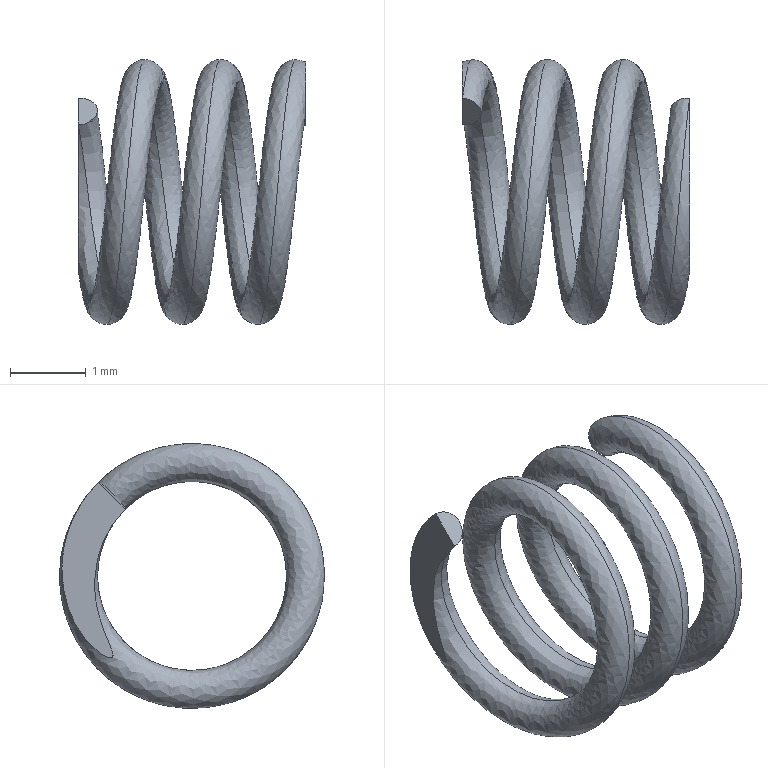Part | SolidWorks | features Helix 1, ICE 1, Sweep 1 | 1 solid | 6 faces | box 3 x 3.5 x 3.5 mm | volume 5.382 mm3 | plane 4 | spline 2
STEP:
#1=CARTESIAN_POINT('',(0.,1.237,1.237));
#2=VERTEX_POINT('',#1);
#3=CARTESIAN_POINT('',(0.,0.8839,0.8839));
#4=VERTEX_POINT('',#3);
#5=CARTESIAN_POINT('',(0.,1.061,1.061));
#6=DIRECTION('',(0.1055,0.7032,-0.7032));
#7=DIRECTION('',(0.,0.7071,0.7071));
#8=AXIS2_PLACEMENT_3D('',#5,#6,#7);
#9=CIRCLE('',#8,0.25);
#10=EDGE_CURVE('',#2,#4,#9,.T.);
#11=ORIENTED_EDGE('',*,*,#10,.T.);
#12=CARTESIAN_POINT('',(3.,0.8839,0.8839));
#13=VERTEX_POINT('',#12);
#14=CARTESIAN_POINT('',(0.,0.8839,0.8839));
#15=CARTESIAN_POINT('',(0.0625,1.25,0.5178));
#16=CARTESIAN_POINT('',(0.125,1.25,0.));
#17=CARTESIAN_POINT('',(0.1875,1.25,-0.5178));
#18=CARTESIAN_POINT('',(0.25,0.8839,-0.8839));
#19=CARTESIAN_POINT('',(0.3125,0.5178,-1.25));
#20=CARTESIAN_POINT('',(0.375,0.,-1.25));
#21=CARTESIAN_POINT('',(0.4375,-0.5178,-1.25));
#22=CARTESIAN_POINT('',(0.5,-0.8839,-0.8839));
#23=CARTESIAN_POINT('',(0.5625,-1.25,-0.5178));
#24=CARTESIAN_POINT('',(0.625,-1.25,0.));
#25=CARTESIAN_POINT('',(0.6875,-1.25,0.5178));
#26=CARTESIAN_POINT('',(0.75,-0.8839,0.8839));
#27=CARTESIAN_POINT('',(0.8125,-0.5178,1.25));
#28=CARTESIAN_POINT('',(0.875,0.,1.25));
#29=CARTESIAN_POINT('',(0.9375,0.5178,1.25));
#30=CARTESIAN_POINT('',(1.,0.8839,0.8839));
#31=CARTESIAN_POINT('',(1.063,1.25,0.5178));
#32=CARTESIAN_POINT('',(1.125,1.25,0.));
#33=CARTESIAN_POINT('',(1.188,1.25,-0.5178));
#34=CARTESIAN_POINT('',(1.25,0.8839,-0.8839));
#35=CARTESIAN_POINT('',(1.313,0.5178,-1.25));
#36=CARTESIAN_POINT('',(1.375,0.,-1.25));
#37=CARTESIAN_POINT('',(1.438,-0.5178,-1.25));
#38=CARTESIAN_POINT('',(1.5,-0.8839,-0.8839));
#39=CARTESIAN_POINT('',(1.562,-1.25,-0.5178));
#40=CARTESIAN_POINT('',(1.625,-1.25,0.));
#41=CARTESIAN_POINT('',(1.688,-1.25,0.5178));
#42=CARTESIAN_POINT('',(1.75,-0.8839,0.8839));
#43=CARTESIAN_POINT('',(1.812,-0.5178,1.25));
#44=CARTESIAN_POINT('',(1.875,0.,1.25));
#45=CARTESIAN_POINT('',(1.938,0.5178,1.25));
#46=CARTESIAN_POINT('',(2.,0.8839,0.8839));
#47=CARTESIAN_POINT('',(2.062,1.25,0.5178));
#48=CARTESIAN_POINT('',(2.125,1.25,0.));
#49=CARTESIAN_POINT('',(2.188,1.25,-0.5178));
#50=CARTESIAN_POINT('',(2.25,0.8839,-0.8839));
#51=CARTESIAN_POINT('',(2.313,0.5178,-1.25));
#52=CARTESIAN_POINT('',(2.375,0.,-1.25));
#53=CARTESIAN_POINT('',(2.438,-0.5178,-1.25));
#54=CARTESIAN_POINT('',(2.5,-0.8839,-0.8839));
#55=CARTESIAN_POINT('',(2.563,-1.25,-0.5178));
#56=CARTESIAN_POINT('',(2.625,-1.25,0.));
#57=CARTESIAN_POINT('',(2.688,-1.25,0.5178));
#58=CARTESIAN_POINT('',(2.75,-0.8839,0.8839));
#59=CARTESIAN_POINT('',(2.812,-0.5178,1.25));
#60=CARTESIAN_POINT('',(2.875,0.,1.25));
#61=CARTESIAN_POINT('',(2.938,0.5178,1.25));
#62=CARTESIAN_POINT('',(3.,0.8839,0.8839));
#63=(BOUNDED_CURVE()B_SPLINE_CURVE(2,(#14,#15,#16,#17,#18,#19,#20,#21,#22,#23,#24,#25,#26,#27,#28,#29,#30,#31,#32,#33,#34,#35,#36,#37,#38,#39,#40,#41,#42,#43,#44,#45,#46,#47,#48,#49,#50,#51,#52,#53,#54,#55,#56,#57,#58,#59,#60,#61,#62),.UNSPECIFIED.,.F.,.T.)B_SPLINE_CURVE_WITH_KNOTS((3,2,2,2,2,2,2,2,2,2,2,2,2,2,2,2,2,2,2,2,2,2,2,2,3),(0.,0.04167,0.08333,0.125,0.1667,0.2083,0.25,0.2917,0.3333,0.375,0.4167,0.4583,0.5,0.5417,0.5833,0.625,0.6667,0.7083,0.75,0.7917,0.8333,0.875,0.9167,0.9583,1.),.UNSPECIFIED.)CURVE()GEOMETRIC_REPRESENTATION_ITEM()RATIONAL_B_SPLINE_CURVE((1.,0.9239,1.,0.9239,1.,0.9239,1.,0.9239,1.,0.9239,1.,0.9239,1.,0.9239,1.,0.9239,1.,0.9239,1.,0.9239,1.,0.9239,1.,0.9239,1.,0.9239,1.,0.9239,1.,0.9239,1.,0.9239,1.,0.9239,1.,0.9239,1.,0.9239,1.,0.9239,1.,0.9239,1.,0.9239,1.,0.9239,1.,0.9239,1.))REPRESENTATION_ITEM(''));
#64=EDGE_CURVE('',#4,#13,#63,.T.);
#65=ORIENTED_EDGE('',*,*,#64,.T.);
#66=CARTESIAN_POINT('',(3.,1.237,1.237));
#67=VERTEX_POINT('',#66);
#68=CARTESIAN_POINT('',(3.,0.8839,0.8839));
#69=CARTESIAN_POINT('',(3.,0.8117,0.956));
#70=CARTESIAN_POINT('',(3.,0.7329,1.019));
#71=CARTESIAN_POINT('',(3.,0.5624,1.126));
#72=CARTESIAN_POINT('',(3.,0.4699,1.171));
#73=CARTESIAN_POINT('',(3.,0.1851,1.273));
#74=CARTESIAN_POINT('',(3.,-0.02075,1.298));
#75=CARTESIAN_POINT('',(3.,-0.3223,1.273));
#76=CARTESIAN_POINT('',(3.,-0.4231,1.255));
#77=CARTESIAN_POINT('',(3.,-0.6187,1.203));
#78=CARTESIAN_POINT('',(3.,-0.7141,1.167));
#79=CARTESIAN_POINT('',(3.,-0.8547,1.108));
#80=CARTESIAN_POINT('',(3.,-0.901,1.087));
#81=CARTESIAN_POINT('',(3.,-0.9719,1.059));
#82=CARTESIAN_POINT('',(3.,-0.9959,1.05));
#83=CARTESIAN_POINT('',(3.,-1.033,1.043));
#84=CARTESIAN_POINT('',(3.,-1.046,1.041));
#85=CARTESIAN_POINT('',(3.,-1.071,1.049));
#86=CARTESIAN_POINT('',(3.,-1.078,1.062));
#87=CARTESIAN_POINT('',(3.,-1.079,1.101));
#88=CARTESIAN_POINT('',(3.,-1.068,1.125));
#89=CARTESIAN_POINT('',(3.,-1.046,1.17));
#90=CARTESIAN_POINT('',(3.,-1.033,1.192));
#91=CARTESIAN_POINT('',(3.,-0.9907,1.254));
#92=CARTESIAN_POINT('',(3.,-0.9577,1.292));
#93=CARTESIAN_POINT('',(3.,-0.8525,1.398));
#94=CARTESIAN_POINT('',(3.,-0.7724,1.46));
#95=CARTESIAN_POINT('',(3.,-0.6013,1.563));
#96=CARTESIAN_POINT('',(3.,-0.5113,1.605));
#97=CARTESIAN_POINT('',(3.,-0.3232,1.669));
#98=CARTESIAN_POINT('',(3.,-0.2247,1.692));
#99=CARTESIAN_POINT('',(3.,-0.02778,1.718));
#100=CARTESIAN_POINT('',(3.,0.07173,1.722));
#101=CARTESIAN_POINT('',(3.,0.3722,1.705));
#102=CARTESIAN_POINT('',(3.,0.5671,1.657));
#103=CARTESIAN_POINT('',(3.,0.9306,1.493));
#104=CARTESIAN_POINT('',(3.,1.096,1.379));
#105=CARTESIAN_POINT('',(3.,1.237,1.237));
#106=B_SPLINE_CURVE_WITH_KNOTS('',3,(#68,#69,#70,#71,#72,#73,#74,#75,#76,#77,#78,#79,#80,#81,#82,#83,#84,#85,#86,#87,#88,#89,#90,#91,#92,#93,#94,#95,#96,#97,#98,#99,#100,#101,#102,#103,#104,#105),.UNSPECIFIED.,.F.,.F.,(4,2,2,2,2,2,2,2,2,2,2,2,2,2,2,2,2,2,4),(0.,0.0003018,0.0006036,0.001207,0.001509,0.001811,0.001962,0.002037,0.002075,0.002113,0.002188,0.002263,0.002414,0.002716,0.003018,0.00332,0.003622,0.004225,0.004829),.UNSPECIFIED.);
#107=EDGE_CURVE('',#13,#67,#106,.T.);
#108=ORIENTED_EDGE('',*,*,#107,.T.);
#109=CARTESIAN_POINT('',(0.,1.237,1.237));
#110=CARTESIAN_POINT('',(0.0625,1.75,0.7249));
#111=CARTESIAN_POINT('',(0.125,1.75,0.));
#112=CARTESIAN_POINT('',(0.1875,1.75,-0.7249));
#113=CARTESIAN_POINT('',(0.25,1.237,-1.237));
#114=CARTESIAN_POINT('',(0.3125,0.7249,-1.75));
#115=CARTESIAN_POINT('',(0.375,0.,-1.75));
#116=CARTESIAN_POINT('',(0.4375,-0.7249,-1.75));
#117=CARTESIAN_POINT('',(0.5,-1.237,-1.237));
#118=CARTESIAN_POINT('',(0.5625,-1.75,-0.7249));
#119=CARTESIAN_POINT('',(0.625,-1.75,0.));
#120=CARTESIAN_POINT('',(0.6875,-1.75,0.7249));
#121=CARTESIAN_POINT('',(0.75,-1.237,1.237));
#122=CARTESIAN_POINT('',(0.8125,-0.7249,1.75));
#123=CARTESIAN_POINT('',(0.875,0.,1.75));
#124=CARTESIAN_POINT('',(0.9375,0.7249,1.75));
#125=CARTESIAN_POINT('',(1.,1.237,1.237));
#126=CARTESIAN_POINT('',(1.063,1.75,0.7249));
#127=CARTESIAN_POINT('',(1.125,1.75,0.));
#128=CARTESIAN_POINT('',(1.188,1.75,-0.7249));
#129=CARTESIAN_POINT('',(1.25,1.237,-1.237));
#130=CARTESIAN_POINT('',(1.313,0.7249,-1.75));
#131=CARTESIAN_POINT('',(1.375,0.,-1.75));
#132=CARTESIAN_POINT('',(1.438,-0.7249,-1.75));
#133=CARTESIAN_POINT('',(1.5,-1.237,-1.237));
#134=CARTESIAN_POINT('',(1.562,-1.75,-0.7249));
#135=CARTESIAN_POINT('',(1.625,-1.75,0.));
#136=CARTESIAN_POINT('',(1.688,-1.75,0.7249));
#137=CARTESIAN_POINT('',(1.75,-1.237,1.237));
#138=CARTESIAN_POINT('',(1.812,-0.7249,1.75));
#139=CARTESIAN_POINT('',(1.875,0.,1.75));
#140=CARTESIAN_POINT('',(1.938,0.7249,1.75));
#141=CARTESIAN_POINT('',(2.,1.237,1.237));
#142=CARTESIAN_POINT('',(2.062,1.75,0.7249));
#143=CARTESIAN_POINT('',(2.125,1.75,0.));
#144=CARTESIAN_POINT('',(2.188,1.75,-0.7249));
#145=CARTESIAN_POINT('',(2.25,1.237,-1.237));
#146=CARTESIAN_POINT('',(2.313,0.7249,-1.75));
#147=CARTESIAN_POINT('',(2.375,0.,-1.75));
#148=CARTESIAN_POINT('',(2.438,-0.7249,-1.75));
#149=CARTESIAN_POINT('',(2.5,-1.237,-1.237));
#150=CARTESIAN_POINT('',(2.563,-1.75,-0.7249));
#151=CARTESIAN_POINT('',(2.625,-1.75,0.));
#152=CARTESIAN_POINT('',(2.688,-1.75,0.7249));
#153=CARTESIAN_POINT('',(2.75,-1.237,1.237));
#154=CARTESIAN_POINT('',(2.812,-0.7249,1.75));
#155=CARTESIAN_POINT('',(2.875,0.,1.75));
#156=CARTESIAN_POINT('',(2.938,0.7249,1.75));
#157=CARTESIAN_POINT('',(3.,1.237,1.237));
#158=(BOUNDED_CURVE()B_SPLINE_CURVE(2,(#109,#110,#111,#112,#113,#114,#115,#116,#117,#118,#119,#120,#121,#122,#123,#124,#125,#126,#127,#128,#129,#130,#131,#132,#133,#134,#135,#136,#137,#138,#139,#140,#141,#142,#143,#144,#145,#146,#147,#148,#149,#150,#151,#152,#153,#154,#155,#156,#157),.UNSPECIFIED.,.F.,.T.)B_SPLINE_CURVE_WITH_KNOTS((3,2,2,2,2,2,2,2,2,2,2,2,2,2,2,2,2,2,2,2,2,2,2,2,3),(0.,0.04167,0.08333,0.125,0.1667,0.2083,0.25,0.2917,0.3333,0.375,0.4167,0.4583,0.5,0.5417,0.5833,0.625,0.6667,0.7083,0.75,0.7917,0.8333,0.875,0.9167,0.9583,1.),.UNSPECIFIED.)CURVE()GEOMETRIC_REPRESENTATION_ITEM()RATIONAL_B_SPLINE_CURVE((1.,0.9239,1.,0.9239,1.,0.9239,1.,0.9239,1.,0.9239,1.,0.9239,1.,0.9239,1.,0.9239,1.,0.9239,1.,0.9239,1.,0.9239,1.,0.9239,1.,0.9239,1.,0.9239,1.,0.9239,1.,0.9239,1.,0.9239,1.,0.9239,1.,0.9239,1.,0.9239,1.,0.9239,1.,0.9239,1.,0.9239,1.,0.9239,1.))REPRESENTATION_ITEM(''));
#159=EDGE_CURVE('',#2,#67,#158,.T.);
#160=ORIENTED_EDGE('',*,*,#159,.F.);
#161=EDGE_LOOP('',(#11,#65,#108,#160));
#162=FACE_OUTER_BOUND('',#161,.T.);
#163=CARTESIAN_POINT('',(0.,1.237,1.237));
#164=CARTESIAN_POINT('',(0.0625,1.75,0.7249));
#165=CARTESIAN_POINT('',(0.125,1.75,0.));
#166=CARTESIAN_POINT('',(0.1875,1.75,-0.7249));
#167=CARTESIAN_POINT('',(0.25,1.237,-1.237));
#168=CARTESIAN_POINT('',(0.3125,0.7249,-1.75));
#169=CARTESIAN_POINT('',(0.375,0.,-1.75));
#170=CARTESIAN_POINT('',(0.4375,-0.7249,-1.75));
#171=CARTESIAN_POINT('',(0.5,-1.237,-1.237));
#172=CARTESIAN_POINT('',(0.5625,-1.75,-0.7249));
#173=CARTESIAN_POINT('',(0.625,-1.75,0.));
#174=CARTESIAN_POINT('',(0.6875,-1.75,0.7249));
#175=CARTESIAN_POINT('',(0.75,-1.237,1.237));
#176=CARTESIAN_POINT('',(0.8125,-0.7249,1.75));
#177=CARTESIAN_POINT('',(0.875,0.,1.75));
#178=CARTESIAN_POINT('',(0.9375,0.7249,1.75));
#179=CARTESIAN_POINT('',(1.,1.237,1.237));
#180=CARTESIAN_POINT('',(1.063,1.75,0.7249));
#181=CARTESIAN_POINT('',(1.125,1.75,0.));
#182=CARTESIAN_POINT('',(1.188,1.75,-0.7249));
#183=CARTESIAN_POINT('',(1.25,1.237,-1.237));
#184=CARTESIAN_POINT('',(1.313,0.7249,-1.75));
#185=CARTESIAN_POINT('',(1.375,0.,-1.75));
#186=CARTESIAN_POINT('',(1.438,-0.7249,-1.75));
#187=CARTESIAN_POINT('',(1.5,-1.237,-1.237));
#188=CARTESIAN_POINT('',(1.562,-1.75,-0.7249));
#189=CARTESIAN_POINT('',(1.625,-1.75,0.));
#190=CARTESIAN_POINT('',(1.688,-1.75,0.7249));
#191=CARTESIAN_POINT('',(1.75,-1.237,1.237));
#192=CARTESIAN_POINT('',(1.813,-0.7249,1.75));
#193=CARTESIAN_POINT('',(1.875,0.,1.75));
#194=CARTESIAN_POINT('',(1.938,0.7249,1.75));
#195=CARTESIAN_POINT('',(2.,1.237,1.237));
#196=CARTESIAN_POINT('',(2.062,1.75,0.7249));
#197=CARTESIAN_POINT('',(2.125,1.75,0.));
#198=CARTESIAN_POINT('',(2.188,1.75,-0.7249));
#199=CARTESIAN_POINT('',(2.25,1.237,-1.237));
#200=CARTESIAN_POINT('',(2.313,0.7249,-1.75));
#201=CARTESIAN_POINT('',(2.375,0.,-1.75));
#202=CARTESIAN_POINT('',(2.438,-0.7249,-1.75));
#203=CARTESIAN_POINT('',(2.5,-1.237,-1.237));
#204=CARTESIAN_POINT('',(2.563,-1.75,-0.7249));
#205=CARTESIAN_POINT('',(2.625,-1.75,0.));
#206=CARTESIAN_POINT('',(2.688,-1.75,0.7249));
#207=CARTESIAN_POINT('',(2.75,-1.237,1.237));
#208=CARTESIAN_POINT('',(2.812,-0.7249,1.75));
#209=CARTESIAN_POINT('',(2.875,0.,1.75));
#210=CARTESIAN_POINT('',(2.938,0.7249,1.75));
#211=CARTESIAN_POINT('',(3.,1.237,1.237));
#212=CARTESIAN_POINT('',(0.4972,1.2,1.275));
#213=CARTESIAN_POINT('',(0.5597,1.728,0.7776));
#214=CARTESIAN_POINT('',(0.6222,1.75,0.05276));
#215=CARTESIAN_POINT('',(0.6847,1.772,-0.6721));
#216=CARTESIAN_POINT('',(0.7472,1.275,-1.2));
#217=CARTESIAN_POINT('',(0.8097,0.7776,-1.728));
#218=CARTESIAN_POINT('',(0.8722,0.05276,-1.75));
#219=CARTESIAN_POINT('',(0.9347,-0.6721,-1.772));
#220=CARTESIAN_POINT('',(0.9972,-1.2,-1.275));
#221=CARTESIAN_POINT('',(1.06,-1.728,-0.7776));
#222=CARTESIAN_POINT('',(1.122,-1.75,-0.05276));
#223=CARTESIAN_POINT('',(1.185,-1.772,0.6721));
#224=CARTESIAN_POINT('',(1.247,-1.275,1.2));
#225=CARTESIAN_POINT('',(1.31,-0.7776,1.728));
#226=CARTESIAN_POINT('',(1.372,-0.05276,1.75));
#227=CARTESIAN_POINT('',(1.435,0.6721,1.772));
#228=CARTESIAN_POINT('',(1.497,1.2,1.275));
#229=CARTESIAN_POINT('',(1.56,1.728,0.7776));
#230=CARTESIAN_POINT('',(1.622,1.75,0.05276));
#231=CARTESIAN_POINT('',(1.685,1.772,-0.6721));
#232=CARTESIAN_POINT('',(1.747,1.275,-1.2));
#233=CARTESIAN_POINT('',(1.81,0.7776,-1.728));
#234=CARTESIAN_POINT('',(1.872,0.05276,-1.75));
#235=CARTESIAN_POINT('',(1.935,-0.6721,-1.772));
#236=CARTESIAN_POINT('',(1.997,-1.2,-1.275));
#237=CARTESIAN_POINT('',(2.06,-1.728,-0.7776));
#238=CARTESIAN_POINT('',(2.122,-1.75,-0.05276));
#239=CARTESIAN_POINT('',(2.185,-1.772,0.6721));
#240=CARTESIAN_POINT('',(2.247,-1.275,1.2));
#241=CARTESIAN_POINT('',(2.31,-0.7776,1.728));
#242=CARTESIAN_POINT('',(2.372,-0.05276,1.75));
#243=CARTESIAN_POINT('',(2.435,0.6721,1.772));
#244=CARTESIAN_POINT('',(2.497,1.2,1.275));
#245=CARTESIAN_POINT('',(2.56,1.728,0.7776));
#246=CARTESIAN_POINT('',(2.622,1.75,0.05276));
#247=CARTESIAN_POINT('',(2.685,1.772,-0.6721));
#248=CARTESIAN_POINT('',(2.747,1.275,-1.2));
#249=CARTESIAN_POINT('',(2.81,0.7776,-1.728));
#250=CARTESIAN_POINT('',(2.872,0.05276,-1.75));
#251=CARTESIAN_POINT('',(2.935,-0.6721,-1.772));
#252=CARTESIAN_POINT('',(2.997,-1.2,-1.275));
#253=CARTESIAN_POINT('',(3.06,-1.728,-0.7776));
#254=CARTESIAN_POINT('',(3.122,-1.75,-0.05276));
#255=CARTESIAN_POINT('',(3.185,-1.772,0.6721));
#256=CARTESIAN_POINT('',(3.247,-1.275,1.2));
#257=CARTESIAN_POINT('',(3.31,-0.7776,1.728));
#258=CARTESIAN_POINT('',(3.372,-0.05276,1.75));
#259=CARTESIAN_POINT('',(3.435,0.6721,1.772));
#260=CARTESIAN_POINT('',(3.497,1.2,1.275));
#261=CARTESIAN_POINT('',(0.4972,0.8466,0.9212));
#262=CARTESIAN_POINT('',(0.5597,1.228,0.5705));
#263=CARTESIAN_POINT('',(0.6222,1.25,0.05276));
#264=CARTESIAN_POINT('',(0.6847,1.272,-0.465));
#265=CARTESIAN_POINT('',(0.7472,0.9212,-0.8466));
#266=CARTESIAN_POINT('',(0.8097,0.5705,-1.228));
#267=CARTESIAN_POINT('',(0.8722,0.05276,-1.25));
#268=CARTESIAN_POINT('',(0.9347,-0.465,-1.272));
#269=CARTESIAN_POINT('',(0.9972,-0.8466,-0.9212));
#270=CARTESIAN_POINT('',(1.06,-1.228,-0.5705));
#271=CARTESIAN_POINT('',(1.122,-1.25,-0.05276));
#272=CARTESIAN_POINT('',(1.185,-1.272,0.465));
#273=CARTESIAN_POINT('',(1.247,-0.9212,0.8466));
#274=CARTESIAN_POINT('',(1.31,-0.5705,1.228));
#275=CARTESIAN_POINT('',(1.372,-0.05276,1.25));
#276=CARTESIAN_POINT('',(1.435,0.465,1.272));
#277=CARTESIAN_POINT('',(1.497,0.8466,0.9212));
#278=CARTESIAN_POINT('',(1.56,1.228,0.5705));
#279=CARTESIAN_POINT('',(1.622,1.25,0.05276));
#280=CARTESIAN_POINT('',(1.685,1.272,-0.465));
#281=CARTESIAN_POINT('',(1.747,0.9212,-0.8466));
#282=CARTESIAN_POINT('',(1.81,0.5705,-1.228));
#283=CARTESIAN_POINT('',(1.872,0.05276,-1.25));
#284=CARTESIAN_POINT('',(1.935,-0.465,-1.272));
#285=CARTESIAN_POINT('',(1.997,-0.8466,-0.9212));
#286=CARTESIAN_POINT('',(2.06,-1.228,-0.5705));
#287=CARTESIAN_POINT('',(2.122,-1.25,-0.05276));
#288=CARTESIAN_POINT('',(2.185,-1.272,0.465));
#289=CARTESIAN_POINT('',(2.247,-0.9212,0.8466));
#290=CARTESIAN_POINT('',(2.31,-0.5705,1.228));
#291=CARTESIAN_POINT('',(2.372,-0.05276,1.25));
#292=CARTESIAN_POINT('',(2.435,0.465,1.272));
#293=CARTESIAN_POINT('',(2.497,0.8466,0.9212));
#294=CARTESIAN_POINT('',(2.56,1.228,0.5705));
#295=CARTESIAN_POINT('',(2.622,1.25,0.05276));
#296=CARTESIAN_POINT('',(2.685,1.272,-0.465));
#297=CARTESIAN_POINT('',(2.747,0.9212,-0.8466));
#298=CARTESIAN_POINT('',(2.81,0.5705,-1.228));
#299=CARTESIAN_POINT('',(2.872,0.05276,-1.25));
#300=CARTESIAN_POINT('',(2.935,-0.465,-1.272));
#301=CARTESIAN_POINT('',(2.997,-0.8466,-0.9212));
#302=CARTESIAN_POINT('',(3.06,-1.228,-0.5705));
#303=CARTESIAN_POINT('',(3.122,-1.25,-0.05276));
#304=CARTESIAN_POINT('',(3.185,-1.272,0.465));
#305=CARTESIAN_POINT('',(3.247,-0.9212,0.8466));
#306=CARTESIAN_POINT('',(3.31,-0.5705,1.228));
#307=CARTESIAN_POINT('',(3.372,-0.05276,1.25));
#308=CARTESIAN_POINT('',(3.435,0.465,1.272));
#309=CARTESIAN_POINT('',(3.497,0.8466,0.9212));
#310=CARTESIAN_POINT('',(0.,0.8839,0.8839));
#311=CARTESIAN_POINT('',(0.0625,1.25,0.5178));
#312=CARTESIAN_POINT('',(0.125,1.25,0.));
#313=CARTESIAN_POINT('',(0.1875,1.25,-0.5178));
#314=CARTESIAN_POINT('',(0.25,0.8839,-0.8839));
#315=CARTESIAN_POINT('',(0.3125,0.5178,-1.25));
#316=CARTESIAN_POINT('',(0.375,0.,-1.25));
#317=CARTESIAN_POINT('',(0.4375,-0.5178,-1.25));
#318=CARTESIAN_POINT('',(0.5,-0.8839,-0.8839));
#319=CARTESIAN_POINT('',(0.5625,-1.25,-0.5178));
#320=CARTESIAN_POINT('',(0.625,-1.25,0.));
#321=CARTESIAN_POINT('',(0.6875,-1.25,0.5178));
#322=CARTESIAN_POINT('',(0.75,-0.8839,0.8839));
#323=CARTESIAN_POINT('',(0.8125,-0.5178,1.25));
#324=CARTESIAN_POINT('',(0.875,0.,1.25));
#325=CARTESIAN_POINT('',(0.9375,0.5178,1.25));
#326=CARTESIAN_POINT('',(1.,0.8839,0.8839));
#327=CARTESIAN_POINT('',(1.063,1.25,0.5178));
#328=CARTESIAN_POINT('',(1.125,1.25,0.));
#329=CARTESIAN_POINT('',(1.188,1.25,-0.5178));
#330=CARTESIAN_POINT('',(1.25,0.8839,-0.8839));
#331=CARTESIAN_POINT('',(1.313,0.5178,-1.25));
#332=CARTESIAN_POINT('',(1.375,0.,-1.25));
#333=CARTESIAN_POINT('',(1.438,-0.5178,-1.25));
#334=CARTESIAN_POINT('',(1.5,-0.8839,-0.8839));
#335=CARTESIAN_POINT('',(1.562,-1.25,-0.5178));
#336=CARTESIAN_POINT('',(1.625,-1.25,0.));
#337=CARTESIAN_POINT('',(1.688,-1.25,0.5178));
#338=CARTESIAN_POINT('',(1.75,-0.8839,0.8839));
#339=CARTESIAN_POINT('',(1.813,-0.5178,1.25));
#340=CARTESIAN_POINT('',(1.875,0.,1.25));
#341=CARTESIAN_POINT('',(1.938,0.5178,1.25));
#342=CARTESIAN_POINT('',(2.,0.8839,0.8839));
#343=CARTESIAN_POINT('',(2.062,1.25,0.5178));
#344=CARTESIAN_POINT('',(2.125,1.25,0.));
#345=CARTESIAN_POINT('',(2.188,1.25,-0.5178));
#346=CARTESIAN_POINT('',(2.25,0.8839,-0.8839));
#347=CARTESIAN_POINT('',(2.313,0.5178,-1.25));
#348=CARTESIAN_POINT('',(2.375,0.,-1.25));
#349=CARTESIAN_POINT('',(2.438,-0.5178,-1.25));
#350=CARTESIAN_POINT('',(2.5,-0.8839,-0.8839));
#351=CARTESIAN_POINT('',(2.563,-1.25,-0.5178));
#352=CARTESIAN_POINT('',(2.625,-1.25,0.));
#353=CARTESIAN_POINT('',(2.688,-1.25,0.5178));
#354=CARTESIAN_POINT('',(2.75,-0.8839,0.8839));
#355=CARTESIAN_POINT('',(2.812,-0.5178,1.25));
#356=CARTESIAN_POINT('',(2.875,0.,1.25));
#357=CARTESIAN_POINT('',(2.938,0.5178,1.25));
#358=CARTESIAN_POINT('',(3.,0.8839,0.8839));
#359=CARTESIAN_POINT('',(-0.4972,0.9212,0.8466));
#360=CARTESIAN_POINT('',(-0.4347,1.272,0.465));
#361=CARTESIAN_POINT('',(-0.3722,1.25,-0.05276));
#362=CARTESIAN_POINT('',(-0.3097,1.228,-0.5705));
#363=CARTESIAN_POINT('',(-0.2472,0.8466,-0.9212));
#364=CARTESIAN_POINT('',(-0.1847,0.465,-1.272));
#365=CARTESIAN_POINT('',(-0.1222,-0.05276,-1.25));
#366=CARTESIAN_POINT('',(-0.05971,-0.5705,-1.228));
#367=CARTESIAN_POINT('',(0.002791,-0.9212,-0.8466));
#368=CARTESIAN_POINT('',(0.06529,-1.272,-0.465));
#369=CARTESIAN_POINT('',(0.1278,-1.25,0.05276));
#370=CARTESIAN_POINT('',(0.1903,-1.228,0.5705));
#371=CARTESIAN_POINT('',(0.2528,-0.8466,0.9212));
#372=CARTESIAN_POINT('',(0.3153,-0.465,1.272));
#373=CARTESIAN_POINT('',(0.3778,0.05276,1.25));
#374=CARTESIAN_POINT('',(0.4403,0.5705,1.228));
#375=CARTESIAN_POINT('',(0.5028,0.9212,0.8466));
#376=CARTESIAN_POINT('',(0.5653,1.272,0.465));
#377=CARTESIAN_POINT('',(0.6278,1.25,-0.05276));
#378=CARTESIAN_POINT('',(0.6903,1.228,-0.5705));
#379=CARTESIAN_POINT('',(0.7528,0.8466,-0.9212));
#380=CARTESIAN_POINT('',(0.8153,0.465,-1.272));
#381=CARTESIAN_POINT('',(0.8778,-0.05276,-1.25));
#382=CARTESIAN_POINT('',(0.9403,-0.5705,-1.228));
#383=CARTESIAN_POINT('',(1.003,-0.9212,-0.8466));
#384=CARTESIAN_POINT('',(1.065,-1.272,-0.465));
#385=CARTESIAN_POINT('',(1.128,-1.25,0.05276));
#386=CARTESIAN_POINT('',(1.19,-1.228,0.5705));
#387=CARTESIAN_POINT('',(1.253,-0.8466,0.9212));
#388=CARTESIAN_POINT('',(1.315,-0.465,1.272));
#389=CARTESIAN_POINT('',(1.378,0.05276,1.25));
#390=CARTESIAN_POINT('',(1.44,0.5705,1.228));
#391=CARTESIAN_POINT('',(1.503,0.9212,0.8466));
#392=CARTESIAN_POINT('',(1.565,1.272,0.465));
#393=CARTESIAN_POINT('',(1.628,1.25,-0.05276));
#394=CARTESIAN_POINT('',(1.69,1.228,-0.5705));
#395=CARTESIAN_POINT('',(1.753,0.8466,-0.9212));
#396=CARTESIAN_POINT('',(1.815,0.465,-1.272));
#397=CARTESIAN_POINT('',(1.878,-0.05276,-1.25));
#398=CARTESIAN_POINT('',(1.94,-0.5705,-1.228));
#399=CARTESIAN_POINT('',(2.003,-0.9212,-0.8466));
#400=CARTESIAN_POINT('',(2.065,-1.272,-0.465));
#401=CARTESIAN_POINT('',(2.128,-1.25,0.05276));
#402=CARTESIAN_POINT('',(2.19,-1.228,0.5705));
#403=CARTESIAN_POINT('',(2.253,-0.8466,0.9212));
#404=CARTESIAN_POINT('',(2.315,-0.465,1.272));
#405=CARTESIAN_POINT('',(2.378,0.05276,1.25));
#406=CARTESIAN_POINT('',(2.44,0.5705,1.228));
#407=CARTESIAN_POINT('',(2.503,0.9212,0.8466));
#408=CARTESIAN_POINT('',(-0.4972,1.275,1.2));
#409=CARTESIAN_POINT('',(-0.4347,1.772,0.6721));
#410=CARTESIAN_POINT('',(-0.3722,1.75,-0.05276));
#411=CARTESIAN_POINT('',(-0.3097,1.728,-0.7776));
#412=CARTESIAN_POINT('',(-0.2472,1.2,-1.275));
#413=CARTESIAN_POINT('',(-0.1847,0.6721,-1.772));
#414=CARTESIAN_POINT('',(-0.1222,-0.05276,-1.75));
#415=CARTESIAN_POINT('',(-0.05971,-0.7776,-1.728));
#416=CARTESIAN_POINT('',(0.002791,-1.275,-1.2));
#417=CARTESIAN_POINT('',(0.06529,-1.772,-0.6721));
#418=CARTESIAN_POINT('',(0.1278,-1.75,0.05276));
#419=CARTESIAN_POINT('',(0.1903,-1.728,0.7776));
#420=CARTESIAN_POINT('',(0.2528,-1.2,1.275));
#421=CARTESIAN_POINT('',(0.3153,-0.6721,1.772));
#422=CARTESIAN_POINT('',(0.3778,0.05276,1.75));
#423=CARTESIAN_POINT('',(0.4403,0.7776,1.728));
#424=CARTESIAN_POINT('',(0.5028,1.275,1.2));
#425=CARTESIAN_POINT('',(0.5653,1.772,0.6721));
#426=CARTESIAN_POINT('',(0.6278,1.75,-0.05276));
#427=CARTESIAN_POINT('',(0.6903,1.728,-0.7776));
#428=CARTESIAN_POINT('',(0.7528,1.2,-1.275));
#429=CARTESIAN_POINT('',(0.8153,0.6721,-1.772));
#430=CARTESIAN_POINT('',(0.8778,-0.05276,-1.75));
#431=CARTESIAN_POINT('',(0.9403,-0.7776,-1.728));
#432=CARTESIAN_POINT('',(1.003,-1.275,-1.2));
#433=CARTESIAN_POINT('',(1.065,-1.772,-0.6721));
#434=CARTESIAN_POINT('',(1.128,-1.75,0.05276));
#435=CARTESIAN_POINT('',(1.19,-1.728,0.7776));
#436=CARTESIAN_POINT('',(1.253,-1.2,1.275));
#437=CARTESIAN_POINT('',(1.315,-0.6721,1.772));
#438=CARTESIAN_POINT('',(1.378,0.05276,1.75));
#439=CARTESIAN_POINT('',(1.44,0.7776,1.728));
#440=CARTESIAN_POINT('',(1.503,1.275,1.2));
#441=CARTESIAN_POINT('',(1.565,1.772,0.6721));
#442=CARTESIAN_POINT('',(1.628,1.75,-0.05276));
#443=CARTESIAN_POINT('',(1.69,1.728,-0.7776));
#444=CARTESIAN_POINT('',(1.753,1.2,-1.275));
#445=CARTESIAN_POINT('',(1.815,0.6721,-1.772));
#446=CARTESIAN_POINT('',(1.878,-0.05276,-1.75));
#447=CARTESIAN_POINT('',(1.94,-0.7776,-1.728));
#448=CARTESIAN_POINT('',(2.003,-1.275,-1.2));
#449=CARTESIAN_POINT('',(2.065,-1.772,-0.6721));
#450=CARTESIAN_POINT('',(2.128,-1.75,0.05276));
#451=CARTESIAN_POINT('',(2.19,-1.728,0.7776));
#452=CARTESIAN_POINT('',(2.253,-1.2,1.275));
#453=CARTESIAN_POINT('',(2.315,-0.6721,1.772));
#454=CARTESIAN_POINT('',(2.378,0.05276,1.75));
#455=CARTESIAN_POINT('',(2.44,0.7776,1.728));
#456=CARTESIAN_POINT('',(2.503,1.275,1.2));
#457=CARTESIAN_POINT('',(0.,1.237,1.237));
#458=CARTESIAN_POINT('',(0.0625,1.75,0.7249));
#459=CARTESIAN_POINT('',(0.125,1.75,0.));
#460=CARTESIAN_POINT('',(0.1875,1.75,-0.7249));
#461=CARTESIAN_POINT('',(0.25,1.237,-1.237));
#462=CARTESIAN_POINT('',(0.3125,0.7249,-1.75));
#463=CARTESIAN_POINT('',(0.375,0.,-1.75));
#464=CARTESIAN_POINT('',(0.4375,-0.7249,-1.75));
#465=CARTESIAN_POINT('',(0.5,-1.237,-1.237));
#466=CARTESIAN_POINT('',(0.5625,-1.75,-0.7249));
#467=CARTESIAN_POINT('',(0.625,-1.75,0.));
#468=CARTESIAN_POINT('',(0.6875,-1.75,0.7249));
#469=CARTESIAN_POINT('',(0.75,-1.237,1.237));
#470=CARTESIAN_POINT('',(0.8125,-0.7249,1.75));
#471=CARTESIAN_POINT('',(0.875,0.,1.75));
#472=CARTESIAN_POINT('',(0.9375,0.7249,1.75));
#473=CARTESIAN_POINT('',(1.,1.237,1.237));
#474=CARTESIAN_POINT('',(1.063,1.75,0.7249));
#475=CARTESIAN_POINT('',(1.125,1.75,0.));
#476=CARTESIAN_POINT('',(1.188,1.75,-0.7249));
#477=CARTESIAN_POINT('',(1.25,1.237,-1.237));
#478=CARTESIAN_POINT('',(1.313,0.7249,-1.75));
#479=CARTESIAN_POINT('',(1.375,0.,-1.75));
#480=CARTESIAN_POINT('',(1.438,-0.7249,-1.75));
#481=CARTESIAN_POINT('',(1.5,-1.237,-1.237));
#482=CARTESIAN_POINT('',(1.562,-1.75,-0.7249));
#483=CARTESIAN_POINT('',(1.625,-1.75,0.));
#484=CARTESIAN_POINT('',(1.688,-1.75,0.7249));
#485=CARTESIAN_POINT('',(1.75,-1.237,1.237));
#486=CARTESIAN_POINT('',(1.813,-0.7249,1.75));
#487=CARTESIAN_POINT('',(1.875,0.,1.75));
#488=CARTESIAN_POINT('',(1.938,0.7249,1.75));
#489=CARTESIAN_POINT('',(2.,1.237,1.237));
#490=CARTESIAN_POINT('',(2.062,1.75,0.7249));
#491=CARTESIAN_POINT('',(2.125,1.75,0.));
#492=CARTESIAN_POINT('',(2.188,1.75,-0.7249));
#493=CARTESIAN_POINT('',(2.25,1.237,-1.237));
#494=CARTESIAN_POINT('',(2.313,0.7249,-1.75));
#495=CARTESIAN_POINT('',(2.375,0.,-1.75));
#496=CARTESIAN_POINT('',(2.438,-0.7249,-1.75));
#497=CARTESIAN_POINT('',(2.5,-1.237,-1.237));
#498=CARTESIAN_POINT('',(2.563,-1.75,-0.7249));
#499=CARTESIAN_POINT('',(2.625,-1.75,0.));
#500=CARTESIAN_POINT('',(2.688,-1.75,0.7249));
#501=CARTESIAN_POINT('',(2.75,-1.237,1.237));
#502=CARTESIAN_POINT('',(2.812,-0.7249,1.75));
#503=CARTESIAN_POINT('',(2.875,0.,1.75));
#504=CARTESIAN_POINT('',(2.938,0.7249,1.75));
#505=CARTESIAN_POINT('',(3.,1.237,1.237));
#506=(BOUNDED_SURFACE()B_SPLINE_SURFACE(3,2,((#163,#164,#165,#166,#167,#168,#169,#170,#171,#172,#173,#174,#175,#176,#177,#178,#179,#180,#181,#182,#183,#184,#185,#186,#187,#188,#189,#190,#191,#192,#193,#194,#195,#196,#197,#198,#199,#200,#201,#202,#203,#204,#205,#206,#207,#208,#209,#210,#211),(#212,#213,#214,#215,#216,#217,#218,#219,#220,#221,#222,#223,#224,#225,#226,#227,#228,#229,#230,#231,#232,#233,#234,#235,#236,#237,#238,#239,#240,#241,#242,#243,#244,#245,#246,#247,#248,#249,#250,#251,#252,#253,#254,#255,#256,#257,#258,#259,#260),(#261,#262,#263,#264,#265,#266,#267,#268,#269,#270,#271,#272,#273,#274,#275,#276,#277,#278,#279,#280,#281,#282,#283,#284,#285,#286,#287,#288,#289,#290,#291,#292,#293,#294,#295,#296,#297,#298,#299,#300,#301,#302,#303,#304,#305,#306,#307,#308,#309),(#310,#311,#312,#313,#314,#315,#316,#317,#318,#319,#320,#321,#322,#323,#324,#325,#326,#327,#328,#329,#330,#331,#332,#333,#334,#335,#336,#337,#338,#339,#340,#341,#342,#343,#344,#345,#346,#347,#348,#349,#350,#351,#352,#353,#354,#355,#356,#357,#358),(#359,#360,#361,#362,#363,#364,#365,#366,#367,#368,#369,#370,#371,#372,#373,#374,#375,#376,#377,#378,#379,#380,#381,#382,#383,#384,#385,#386,#387,#388,#389,#390,#391,#392,#393,#394,#395,#396,#397,#398,#399,#400,#401,#402,#403,#404,#405,#406,#407),(#408,#409,#410,#411,#412,#413,#414,#415,#416,#417,#418,#419,#420,#421,#422,#423,#424,#425,#426,#427,#428,#429,#430,#431,#432,#433,#434,#435,#436,#437,#438,#439,#440,#441,#442,#443,#444,#445,#446,#447,#448,#449,#450,#451,#452,#453,#454,#455,#456),(#457,#458,#459,#460,#461,#462,#463,#464,#465,#466,#467,#468,#469,#470,#471,#472,#473,#474,#475,#476,#477,#478,#479,#480,#481,#482,#483,#484,#485,#486,#487,#488,#489,#490,#491,#492,#493,#494,#495,#496,#497,#498,#499,#500,#501,#502,#503,#504,#505)),.UNSPECIFIED.,.T.,.F.,.T.)B_SPLINE_SURFACE_WITH_KNOTS((4,3,4),(3,2,2,2,2,2,2,2,2,2,2,2,2,2,2,2,2,2,2,2,2,2,2,2,3),(0.,0.5,1.),(0.,0.04167,0.08333,0.125,0.1667,0.2083,0.25,0.2917,0.3333,0.375,0.4167,0.4583,0.5,0.5417,0.5833,0.625,0.6667,0.7083,0.75,0.7917,0.8333,0.875,0.9167,0.9583,1.),.UNSPECIFIED.)GEOMETRIC_REPRESENTATION_ITEM()RATIONAL_B_SPLINE_SURFACE(((1.,0.9239,1.,0.9239,1.,0.9239,1.,0.9239,1.,0.9239,1.,0.9239,1.,0.9239,1.,0.9239,1.,0.9239,1.,0.9239,1.,0.9239,1.,0.9239,1.,0.9239,1.,0.9239,1.,0.9239,1.,0.9239,1.,0.9239,1.,0.9239,1.,0.9239,1.,0.9239,1.,0.9239,1.,0.9239,1.,0.9239,1.,0.9239,1.),(0.3333,0.308,0.3333,0.308,0.3333,0.308,0.3333,0.308,0.3333,0.308,0.3333,0.308,0.3333,0.308,0.3333,0.308,0.3333,0.308,0.3333,0.308,0.3333,0.308,0.3333,0.308,0.3333,0.308,0.3333,0.308,0.3333,0.308,0.3333,0.308,0.3333,0.308,0.3333,0.308,0.3333,0.308,0.3333,0.308,0.3333,0.308,0.3333,0.308,0.3333,0.308,0.3333,0.308,0.3333),(0.3333,0.308,0.3333,0.308,0.3333,0.308,0.3333,0.308,0.3333,0.308,0.3333,0.308,0.3333,0.308,0.3333,0.308,0.3333,0.308,0.3333,0.308,0.3333,0.308,0.3333,0.308,0.3333,0.308,0.3333,0.308,0.3333,0.308,0.3333,0.308,0.3333,0.308,0.3333,0.308,0.3333,0.308,0.3333,0.308,0.3333,0.308,0.3333,0.308,0.3333,0.308,0.3333,0.308,0.3333),(1.,0.9239,1.,0.9239,1.,0.9239,1.,0.9239,1.,0.9239,1.,0.9239,1.,0.9239,1.,0.9239,1.,0.9239,1.,0.9239,1.,0.9239,1.,0.9239,1.,0.9239,1.,0.9239,1.,0.9239,1.,0.9239,1.,0.9239,1.,0.9239,1.,0.9239,1.,0.9239,1.,0.9239,1.,0.9239,1.,0.9239,1.,0.9239,1.),(0.3333,0.308,0.3333,0.308,0.3333,0.308,0.3333,0.308,0.3333,0.308,0.3333,0.308,0.3333,0.308,0.3333,0.308,0.3333,0.308,0.3333,0.308,0.3333,0.308,0.3333,0.308,0.3333,0.308,0.3333,0.308,0.3333,0.308,0.3333,0.308,0.3333,0.308,0.3333,0.308,0.3333,0.308,0.3333,0.308,0.3333,0.308,0.3333,0.308,0.3333,0.308,0.3333,0.308,0.3333),(0.3333,0.308,0.3333,0.308,0.3333,0.308,0.3333,0.308,0.3333,0.308,0.3333,0.308,0.3333,0.308,0.3333,0.308,0.3333,0.308,0.3333,0.308,0.3333,0.308,0.3333,0.308,0.3333,0.308,0.3333,0.308,0.3333,0.308,0.3333,0.308,0.3333,0.308,0.3333,0.308,0.3333,0.308,0.3333,0.308,0.3333,0.308,0.3333,0.308,0.3333,0.308,0.3333,0.308,0.3333),(1.,0.9239,1.,0.9239,1.,0.9239,1.,0.9239,1.,0.9239,1.,0.9239,1.,0.9239,1.,0.9239,1.,0.9239,1.,0.9239,1.,0.9239,1.,0.9239,1.,0.9239,1.,0.9239,1.,0.9239,1.,0.9239,1.,0.9239,1.,0.9239,1.,0.9239,1.,0.9239,1.,0.9239,1.,0.9239,1.,0.9239,1.,0.9239,1.)))REPRESENTATION_ITEM('')SURFACE());
#507=ADVANCED_FACE('',(#162),#506,.T.);
#508=ORIENTED_EDGE('',*,*,#10,.F.);
#509=CARTESIAN_POINT('',(0.,0.8839,0.8839));
#510=DIRECTION('',(0.,-0.7071,-0.7071));
#511=VECTOR('',#510,1000.);
#512=LINE('',#509,#511);
#513=EDGE_CURVE('',#2,#4,#512,.T.);
#514=ORIENTED_EDGE('',*,*,#513,.T.);
#515=EDGE_LOOP('',(#508,#514));
#516=FACE_OUTER_BOUND('',#515,.T.);
#517=CARTESIAN_POINT('',(0.,0.8839,0.8839));
#518=DIRECTION('',(-0.1055,-0.7032,0.7032));
#519=DIRECTION('',(0.,-0.7071,-0.7071));
#520=AXIS2_PLACEMENT_3D('',#517,#518,#519);
#521=PLANE('',#520);
#522=ADVANCED_FACE('',(#516),#521,.T.);
#523=CARTESIAN_POINT('',(3.,0.8839,0.8839));
#524=DIRECTION('',(0.,0.7071,0.7071));
#525=VECTOR('',#524,1000.);
#526=LINE('',#523,#525);
#527=EDGE_CURVE('',#13,#67,#526,.T.);
#528=ORIENTED_EDGE('',*,*,#527,.F.);
#529=CARTESIAN_POINT('',(3.,1.061,1.061));
#530=DIRECTION('',(-0.1055,-0.7032,0.7032));
#531=DIRECTION('',(0.,0.7071,0.7071));
#532=AXIS2_PLACEMENT_3D('',#529,#530,#531);
#533=CIRCLE('',#532,0.25);
#534=EDGE_CURVE('',#67,#13,#533,.T.);
#535=ORIENTED_EDGE('',*,*,#534,.F.);
#536=EDGE_LOOP('',(#528,#535));
#537=FACE_OUTER_BOUND('',#536,.T.);
#538=CARTESIAN_POINT('',(3.,0.8839,0.8839));
#539=DIRECTION('',(-0.1055,-0.7032,0.7032));
#540=DIRECTION('',(0.,-0.7071,-0.7071));
#541=AXIS2_PLACEMENT_3D('',#538,#539,#540);
#542=PLANE('',#541);
#543=ADVANCED_FACE('',(#537),#542,.F.);
#544=ORIENTED_EDGE('',*,*,#64,.F.);
#545=CARTESIAN_POINT('',(0.,0.8839,0.8839));
#546=CARTESIAN_POINT('',(0.,0.956,0.8117));
#547=CARTESIAN_POINT('',(0.,1.019,0.7329));
#548=CARTESIAN_POINT('',(0.,1.126,0.5624));
#549=CARTESIAN_POINT('',(0.,1.171,0.4699));
#550=CARTESIAN_POINT('',(0.,1.273,0.1851));
#551=CARTESIAN_POINT('',(0.,1.298,-0.02075));
#552=CARTESIAN_POINT('',(0.,1.273,-0.3223));
#553=CARTESIAN_POINT('',(0.,1.255,-0.4231));
#554=CARTESIAN_POINT('',(0.,1.203,-0.6187));
#555=CARTESIAN_POINT('',(0.,1.167,-0.7141));
#556=CARTESIAN_POINT('',(0.,1.108,-0.8547));
#557=CARTESIAN_POINT('',(0.,1.087,-0.901));
#558=CARTESIAN_POINT('',(0.,1.059,-0.9719));
#559=CARTESIAN_POINT('',(0.,1.05,-0.9959));
#560=CARTESIAN_POINT('',(0.,1.043,-1.033));
#561=CARTESIAN_POINT('',(0.,1.041,-1.046));
#562=CARTESIAN_POINT('',(0.,1.049,-1.071));
#563=CARTESIAN_POINT('',(0.,1.062,-1.078));
#564=CARTESIAN_POINT('',(0.,1.101,-1.079));
#565=CARTESIAN_POINT('',(0.,1.125,-1.068));
#566=CARTESIAN_POINT('',(0.,1.17,-1.046));
#567=CARTESIAN_POINT('',(0.,1.192,-1.033));
#568=CARTESIAN_POINT('',(0.,1.254,-0.9907));
#569=CARTESIAN_POINT('',(0.,1.292,-0.9577));
#570=CARTESIAN_POINT('',(0.,1.398,-0.8525));
#571=CARTESIAN_POINT('',(0.,1.46,-0.7724));
#572=CARTESIAN_POINT('',(0.,1.563,-0.6013));
#573=CARTESIAN_POINT('',(0.,1.605,-0.5113));
#574=CARTESIAN_POINT('',(0.,1.669,-0.3232));
#575=CARTESIAN_POINT('',(0.,1.692,-0.2247));
#576=CARTESIAN_POINT('',(0.,1.718,-0.02778));
#577=CARTESIAN_POINT('',(0.,1.722,0.07173));
#578=CARTESIAN_POINT('',(0.,1.705,0.3722));
#579=CARTESIAN_POINT('',(0.,1.657,0.5671));
#580=CARTESIAN_POINT('',(0.,1.493,0.9306));
#581=CARTESIAN_POINT('',(0.,1.379,1.096));
#582=CARTESIAN_POINT('',(0.,1.237,1.237));
#583=B_SPLINE_CURVE_WITH_KNOTS('',3,(#545,#546,#547,#548,#549,#550,#551,#552,#553,#554,#555,#556,#557,#558,#559,#560,#561,#562,#563,#564,#565,#566,#567,#568,#569,#570,#571,#572,#573,#574,#575,#576,#577,#578,#579,#580,#581,#582),.UNSPECIFIED.,.F.,.F.,(4,2,2,2,2,2,2,2,2,2,2,2,2,2,2,2,2,2,4),(0.,0.0003018,0.0006036,0.001207,0.001509,0.001811,0.001962,0.002037,0.002075,0.002113,0.002188,0.002263,0.002414,0.002716,0.003018,0.00332,0.003622,0.004225,0.004829),.UNSPECIFIED.);
#584=EDGE_CURVE('',#4,#2,#583,.T.);
#585=ORIENTED_EDGE('',*,*,#584,.T.);
#586=ORIENTED_EDGE('',*,*,#159,.T.);
#587=ORIENTED_EDGE('',*,*,#534,.T.);
#588=EDGE_LOOP('',(#544,#585,#586,#587));
#589=FACE_OUTER_BOUND('',#588,.T.);
#590=CARTESIAN_POINT('',(0.,1.237,1.237));
#591=CARTESIAN_POINT('',(0.0625,1.75,0.7249));
#592=CARTESIAN_POINT('',(0.125,1.75,0.));
#593=CARTESIAN_POINT('',(0.1875,1.75,-0.7249));
#594=CARTESIAN_POINT('',(0.25,1.237,-1.237));
#595=CARTESIAN_POINT('',(0.3125,0.7249,-1.75));
#596=CARTESIAN_POINT('',(0.375,0.,-1.75));
#597=CARTESIAN_POINT('',(0.4375,-0.7249,-1.75));
#598=CARTESIAN_POINT('',(0.5,-1.237,-1.237));
#599=CARTESIAN_POINT('',(0.5625,-1.75,-0.7249));
#600=CARTESIAN_POINT('',(0.625,-1.75,0.));
#601=CARTESIAN_POINT('',(0.6875,-1.75,0.7249));
#602=CARTESIAN_POINT('',(0.75,-1.237,1.237));
#603=CARTESIAN_POINT('',(0.8125,-0.7249,1.75));
#604=CARTESIAN_POINT('',(0.875,0.,1.75));
#605=CARTESIAN_POINT('',(0.9375,0.7249,1.75));
#606=CARTESIAN_POINT('',(1.,1.237,1.237));
#607=CARTESIAN_POINT('',(1.063,1.75,0.7249));
#608=CARTESIAN_POINT('',(1.125,1.75,0.));
#609=CARTESIAN_POINT('',(1.188,1.75,-0.7249));
#610=CARTESIAN_POINT('',(1.25,1.237,-1.237));
#611=CARTESIAN_POINT('',(1.313,0.7249,-1.75));
#612=CARTESIAN_POINT('',(1.375,0.,-1.75));
#613=CARTESIAN_POINT('',(1.438,-0.7249,-1.75));
#614=CARTESIAN_POINT('',(1.5,-1.237,-1.237));
#615=CARTESIAN_POINT('',(1.562,-1.75,-0.7249));
#616=CARTESIAN_POINT('',(1.625,-1.75,0.));
#617=CARTESIAN_POINT('',(1.688,-1.75,0.7249));
#618=CARTESIAN_POINT('',(1.75,-1.237,1.237));
#619=CARTESIAN_POINT('',(1.813,-0.7249,1.75));
#620=CARTESIAN_POINT('',(1.875,0.,1.75));
#621=CARTESIAN_POINT('',(1.938,0.7249,1.75));
#622=CARTESIAN_POINT('',(2.,1.237,1.237));
#623=CARTESIAN_POINT('',(2.062,1.75,0.7249));
#624=CARTESIAN_POINT('',(2.125,1.75,0.));
#625=CARTESIAN_POINT('',(2.188,1.75,-0.7249));
#626=CARTESIAN_POINT('',(2.25,1.237,-1.237));
#627=CARTESIAN_POINT('',(2.313,0.7249,-1.75));
#628=CARTESIAN_POINT('',(2.375,0.,-1.75));
#629=CARTESIAN_POINT('',(2.438,-0.7249,-1.75));
#630=CARTESIAN_POINT('',(2.5,-1.237,-1.237));
#631=CARTESIAN_POINT('',(2.563,-1.75,-0.7249));
#632=CARTESIAN_POINT('',(2.625,-1.75,0.));
#633=CARTESIAN_POINT('',(2.688,-1.75,0.7249));
#634=CARTESIAN_POINT('',(2.75,-1.237,1.237));
#635=CARTESIAN_POINT('',(2.812,-0.7249,1.75));
#636=CARTESIAN_POINT('',(2.875,0.,1.75));
#637=CARTESIAN_POINT('',(2.938,0.7249,1.75));
#638=CARTESIAN_POINT('',(3.,1.237,1.237));
#639=CARTESIAN_POINT('',(0.4972,1.2,1.275));
#640=CARTESIAN_POINT('',(0.5597,1.728,0.7776));
#641=CARTESIAN_POINT('',(0.6222,1.75,0.05276));
#642=CARTESIAN_POINT('',(0.6847,1.772,-0.6721));
#643=CARTESIAN_POINT('',(0.7472,1.275,-1.2));
#644=CARTESIAN_POINT('',(0.8097,0.7776,-1.728));
#645=CARTESIAN_POINT('',(0.8722,0.05276,-1.75));
#646=CARTESIAN_POINT('',(0.9347,-0.6721,-1.772));
#647=CARTESIAN_POINT('',(0.9972,-1.2,-1.275));
#648=CARTESIAN_POINT('',(1.06,-1.728,-0.7776));
#649=CARTESIAN_POINT('',(1.122,-1.75,-0.05276));
#650=CARTESIAN_POINT('',(1.185,-1.772,0.6721));
#651=CARTESIAN_POINT('',(1.247,-1.275,1.2));
#652=CARTESIAN_POINT('',(1.31,-0.7776,1.728));
#653=CARTESIAN_POINT('',(1.372,-0.05276,1.75));
#654=CARTESIAN_POINT('',(1.435,0.6721,1.772));
#655=CARTESIAN_POINT('',(1.497,1.2,1.275));
#656=CARTESIAN_POINT('',(1.56,1.728,0.7776));
#657=CARTESIAN_POINT('',(1.622,1.75,0.05276));
#658=CARTESIAN_POINT('',(1.685,1.772,-0.6721));
#659=CARTESIAN_POINT('',(1.747,1.275,-1.2));
#660=CARTESIAN_POINT('',(1.81,0.7776,-1.728));
#661=CARTESIAN_POINT('',(1.872,0.05276,-1.75));
#662=CARTESIAN_POINT('',(1.935,-0.6721,-1.772));
#663=CARTESIAN_POINT('',(1.997,-1.2,-1.275));
#664=CARTESIAN_POINT('',(2.06,-1.728,-0.7776));
#665=CARTESIAN_POINT('',(2.122,-1.75,-0.05276));
#666=CARTESIAN_POINT('',(2.185,-1.772,0.6721));
#667=CARTESIAN_POINT('',(2.247,-1.275,1.2));
#668=CARTESIAN_POINT('',(2.31,-0.7776,1.728));
#669=CARTESIAN_POINT('',(2.372,-0.05276,1.75));
#670=CARTESIAN_POINT('',(2.435,0.6721,1.772));
#671=CARTESIAN_POINT('',(2.497,1.2,1.275));
#672=CARTESIAN_POINT('',(2.56,1.728,0.7776));
#673=CARTESIAN_POINT('',(2.622,1.75,0.05276));
#674=CARTESIAN_POINT('',(2.685,1.772,-0.6721));
#675=CARTESIAN_POINT('',(2.747,1.275,-1.2));
#676=CARTESIAN_POINT('',(2.81,0.7776,-1.728));
#677=CARTESIAN_POINT('',(2.872,0.05276,-1.75));
#678=CARTESIAN_POINT('',(2.935,-0.6721,-1.772));
#679=CARTESIAN_POINT('',(2.997,-1.2,-1.275));
#680=CARTESIAN_POINT('',(3.06,-1.728,-0.7776));
#681=CARTESIAN_POINT('',(3.122,-1.75,-0.05276));
#682=CARTESIAN_POINT('',(3.185,-1.772,0.6721));
#683=CARTESIAN_POINT('',(3.247,-1.275,1.2));
#684=CARTESIAN_POINT('',(3.31,-0.7776,1.728));
#685=CARTESIAN_POINT('',(3.372,-0.05276,1.75));
#686=CARTESIAN_POINT('',(3.435,0.6721,1.772));
#687=CARTESIAN_POINT('',(3.497,1.2,1.275));
#688=CARTESIAN_POINT('',(0.4972,0.8466,0.9212));
#689=CARTESIAN_POINT('',(0.5597,1.228,0.5705));
#690=CARTESIAN_POINT('',(0.6222,1.25,0.05276));
#691=CARTESIAN_POINT('',(0.6847,1.272,-0.465));
#692=CARTESIAN_POINT('',(0.7472,0.9212,-0.8466));
#693=CARTESIAN_POINT('',(0.8097,0.5705,-1.228));
#694=CARTESIAN_POINT('',(0.8722,0.05276,-1.25));
#695=CARTESIAN_POINT('',(0.9347,-0.465,-1.272));
#696=CARTESIAN_POINT('',(0.9972,-0.8466,-0.9212));
#697=CARTESIAN_POINT('',(1.06,-1.228,-0.5705));
#698=CARTESIAN_POINT('',(1.122,-1.25,-0.05276));
#699=CARTESIAN_POINT('',(1.185,-1.272,0.465));
#700=CARTESIAN_POINT('',(1.247,-0.9212,0.8466));
#701=CARTESIAN_POINT('',(1.31,-0.5705,1.228));
#702=CARTESIAN_POINT('',(1.372,-0.05276,1.25));
#703=CARTESIAN_POINT('',(1.435,0.465,1.272));
#704=CARTESIAN_POINT('',(1.497,0.8466,0.9212));
#705=CARTESIAN_POINT('',(1.56,1.228,0.5705));
#706=CARTESIAN_POINT('',(1.622,1.25,0.05276));
#707=CARTESIAN_POINT('',(1.685,1.272,-0.465));
#708=CARTESIAN_POINT('',(1.747,0.9212,-0.8466));
#709=CARTESIAN_POINT('',(1.81,0.5705,-1.228));
#710=CARTESIAN_POINT('',(1.872,0.05276,-1.25));
#711=CARTESIAN_POINT('',(1.935,-0.465,-1.272));
#712=CARTESIAN_POINT('',(1.997,-0.8466,-0.9212));
#713=CARTESIAN_POINT('',(2.06,-1.228,-0.5705));
#714=CARTESIAN_POINT('',(2.122,-1.25,-0.05276));
#715=CARTESIAN_POINT('',(2.185,-1.272,0.465));
#716=CARTESIAN_POINT('',(2.247,-0.9212,0.8466));
#717=CARTESIAN_POINT('',(2.31,-0.5705,1.228));
#718=CARTESIAN_POINT('',(2.372,-0.05276,1.25));
#719=CARTESIAN_POINT('',(2.435,0.465,1.272));
#720=CARTESIAN_POINT('',(2.497,0.8466,0.9212));
#721=CARTESIAN_POINT('',(2.56,1.228,0.5705));
#722=CARTESIAN_POINT('',(2.622,1.25,0.05276));
#723=CARTESIAN_POINT('',(2.685,1.272,-0.465));
#724=CARTESIAN_POINT('',(2.747,0.9212,-0.8466));
#725=CARTESIAN_POINT('',(2.81,0.5705,-1.228));
#726=CARTESIAN_POINT('',(2.872,0.05276,-1.25));
#727=CARTESIAN_POINT('',(2.935,-0.465,-1.272));
#728=CARTESIAN_POINT('',(2.997,-0.8466,-0.9212));
#729=CARTESIAN_POINT('',(3.06,-1.228,-0.5705));
#730=CARTESIAN_POINT('',(3.122,-1.25,-0.05276));
#731=CARTESIAN_POINT('',(3.185,-1.272,0.465));
#732=CARTESIAN_POINT('',(3.247,-0.9212,0.8466));
#733=CARTESIAN_POINT('',(3.31,-0.5705,1.228));
#734=CARTESIAN_POINT('',(3.372,-0.05276,1.25));
#735=CARTESIAN_POINT('',(3.435,0.465,1.272));
#736=CARTESIAN_POINT('',(3.497,0.8466,0.9212));
#737=CARTESIAN_POINT('',(0.,0.8839,0.8839));
#738=CARTESIAN_POINT('',(0.0625,1.25,0.5178));
#739=CARTESIAN_POINT('',(0.125,1.25,0.));
#740=CARTESIAN_POINT('',(0.1875,1.25,-0.5178));
#741=CARTESIAN_POINT('',(0.25,0.8839,-0.8839));
#742=CARTESIAN_POINT('',(0.3125,0.5178,-1.25));
#743=CARTESIAN_POINT('',(0.375,0.,-1.25));
#744=CARTESIAN_POINT('',(0.4375,-0.5178,-1.25));
#745=CARTESIAN_POINT('',(0.5,-0.8839,-0.8839));
#746=CARTESIAN_POINT('',(0.5625,-1.25,-0.5178));
#747=CARTESIAN_POINT('',(0.625,-1.25,0.));
#748=CARTESIAN_POINT('',(0.6875,-1.25,0.5178));
#749=CARTESIAN_POINT('',(0.75,-0.8839,0.8839));
#750=CARTESIAN_POINT('',(0.8125,-0.5178,1.25));
#751=CARTESIAN_POINT('',(0.875,0.,1.25));
#752=CARTESIAN_POINT('',(0.9375,0.5178,1.25));
#753=CARTESIAN_POINT('',(1.,0.8839,0.8839));
#754=CARTESIAN_POINT('',(1.063,1.25,0.5178));
#755=CARTESIAN_POINT('',(1.125,1.25,0.));
#756=CARTESIAN_POINT('',(1.188,1.25,-0.5178));
#757=CARTESIAN_POINT('',(1.25,0.8839,-0.8839));
#758=CARTESIAN_POINT('',(1.313,0.5178,-1.25));
#759=CARTESIAN_POINT('',(1.375,0.,-1.25));
#760=CARTESIAN_POINT('',(1.438,-0.5178,-1.25));
#761=CARTESIAN_POINT('',(1.5,-0.8839,-0.8839));
#762=CARTESIAN_POINT('',(1.562,-1.25,-0.5178));
#763=CARTESIAN_POINT('',(1.625,-1.25,0.));
#764=CARTESIAN_POINT('',(1.688,-1.25,0.5178));
#765=CARTESIAN_POINT('',(1.75,-0.8839,0.8839));
#766=CARTESIAN_POINT('',(1.813,-0.5178,1.25));
#767=CARTESIAN_POINT('',(1.875,0.,1.25));
#768=CARTESIAN_POINT('',(1.938,0.5178,1.25));
#769=CARTESIAN_POINT('',(2.,0.8839,0.8839));
#770=CARTESIAN_POINT('',(2.062,1.25,0.5178));
#771=CARTESIAN_POINT('',(2.125,1.25,0.));
#772=CARTESIAN_POINT('',(2.188,1.25,-0.5178));
#773=CARTESIAN_POINT('',(2.25,0.8839,-0.8839));
#774=CARTESIAN_POINT('',(2.313,0.5178,-1.25));
#775=CARTESIAN_POINT('',(2.375,0.,-1.25));
#776=CARTESIAN_POINT('',(2.438,-0.5178,-1.25));
#777=CARTESIAN_POINT('',(2.5,-0.8839,-0.8839));
#778=CARTESIAN_POINT('',(2.563,-1.25,-0.5178));
#779=CARTESIAN_POINT('',(2.625,-1.25,0.));
#780=CARTESIAN_POINT('',(2.688,-1.25,0.5178));
#781=CARTESIAN_POINT('',(2.75,-0.8839,0.8839));
#782=CARTESIAN_POINT('',(2.812,-0.5178,1.25));
#783=CARTESIAN_POINT('',(2.875,0.,1.25));
#784=CARTESIAN_POINT('',(2.938,0.5178,1.25));
#785=CARTESIAN_POINT('',(3.,0.8839,0.8839));
#786=CARTESIAN_POINT('',(-0.4972,0.9212,0.8466));
#787=CARTESIAN_POINT('',(-0.4347,1.272,0.465));
#788=CARTESIAN_POINT('',(-0.3722,1.25,-0.05276));
#789=CARTESIAN_POINT('',(-0.3097,1.228,-0.5705));
#790=CARTESIAN_POINT('',(-0.2472,0.8466,-0.9212));
#791=CARTESIAN_POINT('',(-0.1847,0.465,-1.272));
#792=CARTESIAN_POINT('',(-0.1222,-0.05276,-1.25));
#793=CARTESIAN_POINT('',(-0.05971,-0.5705,-1.228));
#794=CARTESIAN_POINT('',(0.002791,-0.9212,-0.8466));
#795=CARTESIAN_POINT('',(0.06529,-1.272,-0.465));
#796=CARTESIAN_POINT('',(0.1278,-1.25,0.05276));
#797=CARTESIAN_POINT('',(0.1903,-1.228,0.5705));
#798=CARTESIAN_POINT('',(0.2528,-0.8466,0.9212));
#799=CARTESIAN_POINT('',(0.3153,-0.465,1.272));
#800=CARTESIAN_POINT('',(0.3778,0.05276,1.25));
#801=CARTESIAN_POINT('',(0.4403,0.5705,1.228));
#802=CARTESIAN_POINT('',(0.5028,0.9212,0.8466));
#803=CARTESIAN_POINT('',(0.5653,1.272,0.465));
#804=CARTESIAN_POINT('',(0.6278,1.25,-0.05276));
#805=CARTESIAN_POINT('',(0.6903,1.228,-0.5705));
#806=CARTESIAN_POINT('',(0.7528,0.8466,-0.9212));
#807=CARTESIAN_POINT('',(0.8153,0.465,-1.272));
#808=CARTESIAN_POINT('',(0.8778,-0.05276,-1.25));
#809=CARTESIAN_POINT('',(0.9403,-0.5705,-1.228));
#810=CARTESIAN_POINT('',(1.003,-0.9212,-0.8466));
#811=CARTESIAN_POINT('',(1.065,-1.272,-0.465));
#812=CARTESIAN_POINT('',(1.128,-1.25,0.05276));
#813=CARTESIAN_POINT('',(1.19,-1.228,0.5705));
#814=CARTESIAN_POINT('',(1.253,-0.8466,0.9212));
#815=CARTESIAN_POINT('',(1.315,-0.465,1.272));
#816=CARTESIAN_POINT('',(1.378,0.05276,1.25));
#817=CARTESIAN_POINT('',(1.44,0.5705,1.228));
#818=CARTESIAN_POINT('',(1.503,0.9212,0.8466));
#819=CARTESIAN_POINT('',(1.565,1.272,0.465));
#820=CARTESIAN_POINT('',(1.628,1.25,-0.05276));
#821=CARTESIAN_POINT('',(1.69,1.228,-0.5705));
#822=CARTESIAN_POINT('',(1.753,0.8466,-0.9212));
#823=CARTESIAN_POINT('',(1.815,0.465,-1.272));
#824=CARTESIAN_POINT('',(1.878,-0.05276,-1.25));
#825=CARTESIAN_POINT('',(1.94,-0.5705,-1.228));
#826=CARTESIAN_POINT('',(2.003,-0.9212,-0.8466));
#827=CARTESIAN_POINT('',(2.065,-1.272,-0.465));
#828=CARTESIAN_POINT('',(2.128,-1.25,0.05276));
#829=CARTESIAN_POINT('',(2.19,-1.228,0.5705));
#830=CARTESIAN_POINT('',(2.253,-0.8466,0.9212));
#831=CARTESIAN_POINT('',(2.315,-0.465,1.272));
#832=CARTESIAN_POINT('',(2.378,0.05276,1.25));
#833=CARTESIAN_POINT('',(2.44,0.5705,1.228));
#834=CARTESIAN_POINT('',(2.503,0.9212,0.8466));
#835=CARTESIAN_POINT('',(-0.4972,1.275,1.2));
#836=CARTESIAN_POINT('',(-0.4347,1.772,0.6721));
#837=CARTESIAN_POINT('',(-0.3722,1.75,-0.05276));
#838=CARTESIAN_POINT('',(-0.3097,1.728,-0.7776));
#839=CARTESIAN_POINT('',(-0.2472,1.2,-1.275));
#840=CARTESIAN_POINT('',(-0.1847,0.6721,-1.772));
#841=CARTESIAN_POINT('',(-0.1222,-0.05276,-1.75));
#842=CARTESIAN_POINT('',(-0.05971,-0.7776,-1.728));
#843=CARTESIAN_POINT('',(0.002791,-1.275,-1.2));
#844=CARTESIAN_POINT('',(0.06529,-1.772,-0.6721));
#845=CARTESIAN_POINT('',(0.1278,-1.75,0.05276));
#846=CARTESIAN_POINT('',(0.1903,-1.728,0.7776));
#847=CARTESIAN_POINT('',(0.2528,-1.2,1.275));
#848=CARTESIAN_POINT('',(0.3153,-0.6721,1.772));
#849=CARTESIAN_POINT('',(0.3778,0.05276,1.75));
#850=CARTESIAN_POINT('',(0.4403,0.7776,1.728));
#851=CARTESIAN_POINT('',(0.5028,1.275,1.2));
#852=CARTESIAN_POINT('',(0.5653,1.772,0.6721));
#853=CARTESIAN_POINT('',(0.6278,1.75,-0.05276));
#854=CARTESIAN_POINT('',(0.6903,1.728,-0.7776));
#855=CARTESIAN_POINT('',(0.7528,1.2,-1.275));
#856=CARTESIAN_POINT('',(0.8153,0.6721,-1.772));
#857=CARTESIAN_POINT('',(0.8778,-0.05276,-1.75));
#858=CARTESIAN_POINT('',(0.9403,-0.7776,-1.728));
#859=CARTESIAN_POINT('',(1.003,-1.275,-1.2));
#860=CARTESIAN_POINT('',(1.065,-1.772,-0.6721));
#861=CARTESIAN_POINT('',(1.128,-1.75,0.05276));
#862=CARTESIAN_POINT('',(1.19,-1.728,0.7776));
#863=CARTESIAN_POINT('',(1.253,-1.2,1.275));
#864=CARTESIAN_POINT('',(1.315,-0.6721,1.772));
#865=CARTESIAN_POINT('',(1.378,0.05276,1.75));
#866=CARTESIAN_POINT('',(1.44,0.7776,1.728));
#867=CARTESIAN_POINT('',(1.503,1.275,1.2));
#868=CARTESIAN_POINT('',(1.565,1.772,0.6721));
#869=CARTESIAN_POINT('',(1.628,1.75,-0.05276));
#870=CARTESIAN_POINT('',(1.69,1.728,-0.7776));
#871=CARTESIAN_POINT('',(1.753,1.2,-1.275));
#872=CARTESIAN_POINT('',(1.815,0.6721,-1.772));
#873=CARTESIAN_POINT('',(1.878,-0.05276,-1.75));
#874=CARTESIAN_POINT('',(1.94,-0.7776,-1.728));
#875=CARTESIAN_POINT('',(2.003,-1.275,-1.2));
#876=CARTESIAN_POINT('',(2.065,-1.772,-0.6721));
#877=CARTESIAN_POINT('',(2.128,-1.75,0.05276));
#878=CARTESIAN_POINT('',(2.19,-1.728,0.7776));
#879=CARTESIAN_POINT('',(2.253,-1.2,1.275));
#880=CARTESIAN_POINT('',(2.315,-0.6721,1.772));
#881=CARTESIAN_POINT('',(2.378,0.05276,1.75));
#882=CARTESIAN_POINT('',(2.44,0.7776,1.728));
#883=CARTESIAN_POINT('',(2.503,1.275,1.2));
#884=CARTESIAN_POINT('',(0.,1.237,1.237));
#885=CARTESIAN_POINT('',(0.0625,1.75,0.7249));
#886=CARTESIAN_POINT('',(0.125,1.75,0.));
#887=CARTESIAN_POINT('',(0.1875,1.75,-0.7249));
#888=CARTESIAN_POINT('',(0.25,1.237,-1.237));
#889=CARTESIAN_POINT('',(0.3125,0.7249,-1.75));
#890=CARTESIAN_POINT('',(0.375,0.,-1.75));
#891=CARTESIAN_POINT('',(0.4375,-0.7249,-1.75));
#892=CARTESIAN_POINT('',(0.5,-1.237,-1.237));
#893=CARTESIAN_POINT('',(0.5625,-1.75,-0.7249));
#894=CARTESIAN_POINT('',(0.625,-1.75,0.));
#895=CARTESIAN_POINT('',(0.6875,-1.75,0.7249));
#896=CARTESIAN_POINT('',(0.75,-1.237,1.237));
#897=CARTESIAN_POINT('',(0.8125,-0.7249,1.75));
#898=CARTESIAN_POINT('',(0.875,0.,1.75));
#899=CARTESIAN_POINT('',(0.9375,0.7249,1.75));
#900=CARTESIAN_POINT('',(1.,1.237,1.237));
#901=CARTESIAN_POINT('',(1.063,1.75,0.7249));
#902=CARTESIAN_POINT('',(1.125,1.75,0.));
#903=CARTESIAN_POINT('',(1.188,1.75,-0.7249));
#904=CARTESIAN_POINT('',(1.25,1.237,-1.237));
#905=CARTESIAN_POINT('',(1.313,0.7249,-1.75));
#906=CARTESIAN_POINT('',(1.375,0.,-1.75));
#907=CARTESIAN_POINT('',(1.438,-0.7249,-1.75));
#908=CARTESIAN_POINT('',(1.5,-1.237,-1.237));
#909=CARTESIAN_POINT('',(1.562,-1.75,-0.7249));
#910=CARTESIAN_POINT('',(1.625,-1.75,0.));
#911=CARTESIAN_POINT('',(1.688,-1.75,0.7249));
#912=CARTESIAN_POINT('',(1.75,-1.237,1.237));
#913=CARTESIAN_POINT('',(1.813,-0.7249,1.75));
#914=CARTESIAN_POINT('',(1.875,0.,1.75));
#915=CARTESIAN_POINT('',(1.938,0.7249,1.75));
#916=CARTESIAN_POINT('',(2.,1.237,1.237));
#917=CARTESIAN_POINT('',(2.062,1.75,0.7249));
#918=CARTESIAN_POINT('',(2.125,1.75,0.));
#919=CARTESIAN_POINT('',(2.188,1.75,-0.7249));
#920=CARTESIAN_POINT('',(2.25,1.237,-1.237));
#921=CARTESIAN_POINT('',(2.313,0.7249,-1.75));
#922=CARTESIAN_POINT('',(2.375,0.,-1.75));
#923=CARTESIAN_POINT('',(2.438,-0.7249,-1.75));
#924=CARTESIAN_POINT('',(2.5,-1.237,-1.237));
#925=CARTESIAN_POINT('',(2.563,-1.75,-0.7249));
#926=CARTESIAN_POINT('',(2.625,-1.75,0.));
#927=CARTESIAN_POINT('',(2.688,-1.75,0.7249));
#928=CARTESIAN_POINT('',(2.75,-1.237,1.237));
#929=CARTESIAN_POINT('',(2.812,-0.7249,1.75));
#930=CARTESIAN_POINT('',(2.875,0.,1.75));
#931=CARTESIAN_POINT('',(2.938,0.7249,1.75));
#932=CARTESIAN_POINT('',(3.,1.237,1.237));
#933=(BOUNDED_SURFACE()B_SPLINE_SURFACE(3,2,((#590,#591,#592,#593,#594,#595,#596,#597,#598,#599,#600,#601,#602,#603,#604,#605,#606,#607,#608,#609,#610,#611,#612,#613,#614,#615,#616,#617,#618,#619,#620,#621,#622,#623,#624,#625,#626,#627,#628,#629,#630,#631,#632,#633,#634,#635,#636,#637,#638),(#639,#640,#641,#642,#643,#644,#645,#646,#647,#648,#649,#650,#651,#652,#653,#654,#655,#656,#657,#658,#659,#660,#661,#662,#663,#664,#665,#666,#667,#668,#669,#670,#671,#672,#673,#674,#675,#676,#677,#678,#679,#680,#681,#682,#683,#684,#685,#686,#687),(#688,#689,#690,#691,#692,#693,#694,#695,#696,#697,#698,#699,#700,#701,#702,#703,#704,#705,#706,#707,#708,#709,#710,#711,#712,#713,#714,#715,#716,#717,#718,#719,#720,#721,#722,#723,#724,#725,#726,#727,#728,#729,#730,#731,#732,#733,#734,#735,#736),(#737,#738,#739,#740,#741,#742,#743,#744,#745,#746,#747,#748,#749,#750,#751,#752,#753,#754,#755,#756,#757,#758,#759,#760,#761,#762,#763,#764,#765,#766,#767,#768,#769,#770,#771,#772,#773,#774,#775,#776,#777,#778,#779,#780,#781,#782,#783,#784,#785),(#786,#787,#788,#789,#790,#791,#792,#793,#794,#795,#796,#797,#798,#799,#800,#801,#802,#803,#804,#805,#806,#807,#808,#809,#810,#811,#812,#813,#814,#815,#816,#817,#818,#819,#820,#821,#822,#823,#824,#825,#826,#827,#828,#829,#830,#831,#832,#833,#834),(#835,#836,#837,#838,#839,#840,#841,#842,#843,#844,#845,#846,#847,#848,#849,#850,#851,#852,#853,#854,#855,#856,#857,#858,#859,#860,#861,#862,#863,#864,#865,#866,#867,#868,#869,#870,#871,#872,#873,#874,#875,#876,#877,#878,#879,#880,#881,#882,#883),(#884,#885,#886,#887,#888,#889,#890,#891,#892,#893,#894,#895,#896,#897,#898,#899,#900,#901,#902,#903,#904,#905,#906,#907,#908,#909,#910,#911,#912,#913,#914,#915,#916,#917,#918,#919,#920,#921,#922,#923,#924,#925,#926,#927,#928,#929,#930,#931,#932)),.UNSPECIFIED.,.T.,.F.,.T.)B_SPLINE_SURFACE_WITH_KNOTS((4,3,4),(3,2,2,2,2,2,2,2,2,2,2,2,2,2,2,2,2,2,2,2,2,2,2,2,3),(0.,0.5,1.),(0.,0.04167,0.08333,0.125,0.1667,0.2083,0.25,0.2917,0.3333,0.375,0.4167,0.4583,0.5,0.5417,0.5833,0.625,0.6667,0.7083,0.75,0.7917,0.8333,0.875,0.9167,0.9583,1.),.UNSPECIFIED.)GEOMETRIC_REPRESENTATION_ITEM()RATIONAL_B_SPLINE_SURFACE(((1.,0.9239,1.,0.9239,1.,0.9239,1.,0.9239,1.,0.9239,1.,0.9239,1.,0.9239,1.,0.9239,1.,0.9239,1.,0.9239,1.,0.9239,1.,0.9239,1.,0.9239,1.,0.9239,1.,0.9239,1.,0.9239,1.,0.9239,1.,0.9239,1.,0.9239,1.,0.9239,1.,0.9239,1.,0.9239,1.,0.9239,1.,0.9239,1.),(0.3333,0.308,0.3333,0.308,0.3333,0.308,0.3333,0.308,0.3333,0.308,0.3333,0.308,0.3333,0.308,0.3333,0.308,0.3333,0.308,0.3333,0.308,0.3333,0.308,0.3333,0.308,0.3333,0.308,0.3333,0.308,0.3333,0.308,0.3333,0.308,0.3333,0.308,0.3333,0.308,0.3333,0.308,0.3333,0.308,0.3333,0.308,0.3333,0.308,0.3333,0.308,0.3333,0.308,0.3333),(0.3333,0.308,0.3333,0.308,0.3333,0.308,0.3333,0.308,0.3333,0.308,0.3333,0.308,0.3333,0.308,0.3333,0.308,0.3333,0.308,0.3333,0.308,0.3333,0.308,0.3333,0.308,0.3333,0.308,0.3333,0.308,0.3333,0.308,0.3333,0.308,0.3333,0.308,0.3333,0.308,0.3333,0.308,0.3333,0.308,0.3333,0.308,0.3333,0.308,0.3333,0.308,0.3333,0.308,0.3333),(1.,0.9239,1.,0.9239,1.,0.9239,1.,0.9239,1.,0.9239,1.,0.9239,1.,0.9239,1.,0.9239,1.,0.9239,1.,0.9239,1.,0.9239,1.,0.9239,1.,0.9239,1.,0.9239,1.,0.9239,1.,0.9239,1.,0.9239,1.,0.9239,1.,0.9239,1.,0.9239,1.,0.9239,1.,0.9239,1.,0.9239,1.,0.9239,1.),(0.3333,0.308,0.3333,0.308,0.3333,0.308,0.3333,0.308,0.3333,0.308,0.3333,0.308,0.3333,0.308,0.3333,0.308,0.3333,0.308,0.3333,0.308,0.3333,0.308,0.3333,0.308,0.3333,0.308,0.3333,0.308,0.3333,0.308,0.3333,0.308,0.3333,0.308,0.3333,0.308,0.3333,0.308,0.3333,0.308,0.3333,0.308,0.3333,0.308,0.3333,0.308,0.3333,0.308,0.3333),(0.3333,0.308,0.3333,0.308,0.3333,0.308,0.3333,0.308,0.3333,0.308,0.3333,0.308,0.3333,0.308,0.3333,0.308,0.3333,0.308,0.3333,0.308,0.3333,0.308,0.3333,0.308,0.3333,0.308,0.3333,0.308,0.3333,0.308,0.3333,0.308,0.3333,0.308,0.3333,0.308,0.3333,0.308,0.3333,0.308,0.3333,0.308,0.3333,0.308,0.3333,0.308,0.3333,0.308,0.3333),(1.,0.9239,1.,0.9239,1.,0.9239,1.,0.9239,1.,0.9239,1.,0.9239,1.,0.9239,1.,0.9239,1.,0.9239,1.,0.9239,1.,0.9239,1.,0.9239,1.,0.9239,1.,0.9239,1.,0.9239,1.,0.9239,1.,0.9239,1.,0.9239,1.,0.9239,1.,0.9239,1.,0.9239,1.,0.9239,1.,0.9239,1.,0.9239,1.)))REPRESENTATION_ITEM('')SURFACE());
#934=ADVANCED_FACE('',(#589),#933,.T.);
#935=ORIENTED_EDGE('',*,*,#584,.F.);
#936=ORIENTED_EDGE('',*,*,#513,.F.);
#937=EDGE_LOOP('',(#935,#936));
#938=FACE_OUTER_BOUND('',#937,.T.);
#939=CARTESIAN_POINT('',(0.,-2.727,-1.755));
#940=DIRECTION('',(-1.,0.,0.));
#941=DIRECTION('',(0.,0.,1.));
#942=AXIS2_PLACEMENT_3D('',#939,#940,#941);
#943=PLANE('',#942);
#944=ADVANCED_FACE('',(#938),#943,.T.);
#945=ORIENTED_EDGE('',*,*,#527,.T.);
#946=ORIENTED_EDGE('',*,*,#107,.F.);
#947=EDGE_LOOP('',(#945,#946));
#948=FACE_OUTER_BOUND('',#947,.T.);
#949=CARTESIAN_POINT('',(3.,-2.727,-1.755));
#950=DIRECTION('',(1.,0.,0.));
#951=DIRECTION('',(0.,0.,-1.));
#952=AXIS2_PLACEMENT_3D('',#949,#950,#951);
#953=PLANE('',#952);
#954=ADVANCED_FACE('',(#948),#953,.T.);
#955=CLOSED_SHELL('',(#507,#522,#543,#934,#944,#954));
#956=MANIFOLD_SOLID_BREP('',#955);
#957=CARTESIAN_POINT('',(0.,0.,0.));
#958=DIRECTION('',(0.,0.,1.));
#959=DIRECTION('',(1.,0.,0.));
#960=AXIS2_PLACEMENT_3D('',#957,#958,#959);
#961=(LENGTH_UNIT()NAMED_UNIT(*)SI_UNIT(.MILLI.,.METRE.));
#962=UNCERTAINTY_MEASURE_WITH_UNIT(LENGTH_MEASURE(0.00001),#961,'','');
#963=(NAMED_UNIT(*)PLANE_ANGLE_UNIT()SI_UNIT($,.RADIAN.));
#964=(NAMED_UNIT(*)SI_UNIT($,.STERADIAN.)SOLID_ANGLE_UNIT());
#965=(GEOMETRIC_REPRESENTATION_CONTEXT(3)GLOBAL_UNCERTAINTY_ASSIGNED_CONTEXT((#962))GLOBAL_UNIT_ASSIGNED_CONTEXT((#961,#963,#964))REPRESENTATION_CONTEXT('',''));
#966=ADVANCED_BREP_SHAPE_REPRESENTATION('',(#956,#960),#965);